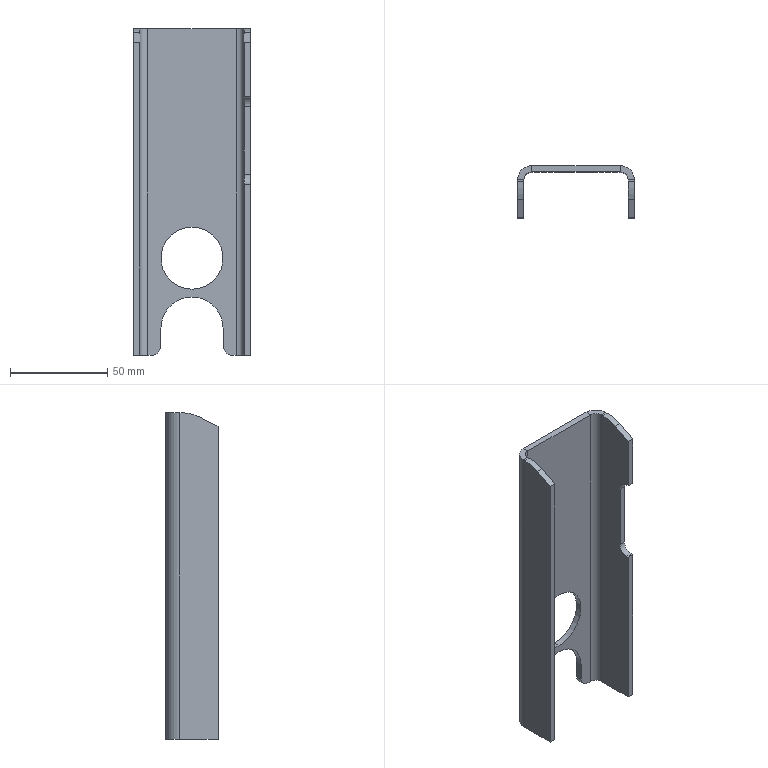Part | SolidWorks | features ICE 3, Fillet 2, FlatPattern 1, SMBaseFlange 1, SheetMetal 1, UnFold 1 | 1 solid | 41 faces | box 60 x 26.8 x 168.2 mm | volume 48634 mm3 | plane 27 | cylinder 14 | commonest cylinder face diameters 10 x4 32 x4 8 x2 14.4 x2 40 x2
STEP:
#1=CARTESIAN_POINT('',(0.,-3.2,34.));
#2=VERTEX_POINT('',#1);
#3=CARTESIAN_POINT('',(0.,-3.2,66.));
#4=VERTEX_POINT('',#3);
#5=CARTESIAN_POINT('',(0.,-3.2,50.));
#6=DIRECTION('',(0.,1.,0.));
#7=DIRECTION('',(0.,0.,1.));
#8=AXIS2_PLACEMENT_3D('',#5,#6,#7);
#9=CIRCLE('',#8,16.);
#10=EDGE_CURVE('',#2,#4,#9,.T.);
#11=ORIENTED_EDGE('',*,*,#10,.F.);
#12=CARTESIAN_POINT('',(0.,0.,34.));
#13=VERTEX_POINT('',#12);
#14=CARTESIAN_POINT('',(0.,-3.2,34.));
#15=DIRECTION('',(0.,1.,0.));
#16=VECTOR('',#15,1000.);
#17=LINE('',#14,#16);
#18=EDGE_CURVE('',#2,#13,#17,.T.);
#19=ORIENTED_EDGE('',*,*,#18,.T.);
#20=CARTESIAN_POINT('',(0.,0.,66.));
#21=VERTEX_POINT('',#20);
#22=CARTESIAN_POINT('',(0.,0.,50.));
#23=DIRECTION('',(0.,1.,0.));
#24=DIRECTION('',(0.,0.,1.));
#25=AXIS2_PLACEMENT_3D('',#22,#23,#24);
#26=CIRCLE('',#25,16.);
#27=EDGE_CURVE('',#13,#21,#26,.T.);
#28=ORIENTED_EDGE('',*,*,#27,.T.);
#29=CARTESIAN_POINT('',(0.,-3.2,66.));
#30=DIRECTION('',(0.,1.,0.));
#31=VECTOR('',#30,1000.);
#32=LINE('',#29,#31);
#33=EDGE_CURVE('',#4,#21,#32,.T.);
#34=ORIENTED_EDGE('',*,*,#33,.F.);
#35=EDGE_LOOP('',(#11,#19,#28,#34));
#36=FACE_OUTER_BOUND('',#35,.T.);
#37=CARTESIAN_POINT('',(0.,-3.2,50.));
#38=DIRECTION('',(0.,1.,0.));
#39=DIRECTION('',(0.,0.,1.));
#40=AXIS2_PLACEMENT_3D('',#37,#38,#39);
#41=CYLINDRICAL_SURFACE('',#40,16.);
#42=ADVANCED_FACE('',(#36),#41,.F.);
#43=CARTESIAN_POINT('',(0.,-3.2,30.));
#44=VERTEX_POINT('',#43);
#45=CARTESIAN_POINT('',(16.,-3.2,14.));
#46=VERTEX_POINT('',#45);
#47=CARTESIAN_POINT('',(0.,-3.2,14.));
#48=DIRECTION('',(0.,1.,0.));
#49=DIRECTION('',(0.,0.,1.));
#50=AXIS2_PLACEMENT_3D('',#47,#48,#49);
#51=CIRCLE('',#50,16.);
#52=EDGE_CURVE('',#44,#46,#51,.T.);
#53=ORIENTED_EDGE('',*,*,#52,.F.);
#54=CARTESIAN_POINT('',(0.,0.,30.));
#55=VERTEX_POINT('',#54);
#56=CARTESIAN_POINT('',(0.,-3.2,30.));
#57=DIRECTION('',(0.,1.,0.));
#58=VECTOR('',#57,1000.);
#59=LINE('',#56,#58);
#60=EDGE_CURVE('',#44,#55,#59,.T.);
#61=ORIENTED_EDGE('',*,*,#60,.T.);
#62=CARTESIAN_POINT('',(16.,0.,14.));
#63=VERTEX_POINT('',#62);
#64=CARTESIAN_POINT('',(0.,0.,14.));
#65=DIRECTION('',(0.,1.,0.));
#66=DIRECTION('',(0.,0.,1.));
#67=AXIS2_PLACEMENT_3D('',#64,#65,#66);
#68=CIRCLE('',#67,16.);
#69=EDGE_CURVE('',#55,#63,#68,.T.);
#70=ORIENTED_EDGE('',*,*,#69,.T.);
#71=CARTESIAN_POINT('',(16.,-3.2,14.));
#72=DIRECTION('',(0.,1.,0.));
#73=VECTOR('',#72,1000.);
#74=LINE('',#71,#73);
#75=EDGE_CURVE('',#46,#63,#74,.T.);
#76=ORIENTED_EDGE('',*,*,#75,.F.);
#77=EDGE_LOOP('',(#53,#61,#70,#76));
#78=FACE_OUTER_BOUND('',#77,.T.);
#79=CARTESIAN_POINT('',(0.,-3.2,14.));
#80=DIRECTION('',(0.,1.,0.));
#81=DIRECTION('',(0.,0.,1.));
#82=AXIS2_PLACEMENT_3D('',#79,#80,#81);
#83=CYLINDRICAL_SURFACE('',#82,16.);
#84=ADVANCED_FACE('',(#78),#83,.F.);
#85=CARTESIAN_POINT('',(26.8,-26.8,133.2));
#86=VERTEX_POINT('',#85);
#87=CARTESIAN_POINT('',(30.,-26.8,133.2));
#88=VERTEX_POINT('',#87);
#89=CARTESIAN_POINT('',(26.8,-26.8,133.2));
#90=DIRECTION('',(1.,0.,0.));
#91=VECTOR('',#90,1000.);
#92=LINE('',#89,#91);
#93=EDGE_CURVE('',#86,#88,#92,.T.);
#94=ORIENTED_EDGE('',*,*,#93,.T.);
#95=CARTESIAN_POINT('',(30.,-26.8,161.2));
#96=VERTEX_POINT('',#95);
#97=CARTESIAN_POINT('',(30.,-26.8,168.2));
#98=DIRECTION('',(0.,0.,-1.));
#99=VECTOR('',#98,1000.);
#100=LINE('',#97,#99);
#101=EDGE_CURVE('',#96,#88,#100,.T.);
#102=ORIENTED_EDGE('',*,*,#101,.F.);
#103=CARTESIAN_POINT('',(26.8,-26.8,161.2));
#104=VERTEX_POINT('',#103);
#105=CARTESIAN_POINT('',(-30.,-26.8,161.2));
#106=DIRECTION('',(1.,0.,0.));
#107=VECTOR('',#106,1000.);
#108=LINE('',#105,#107);
#109=EDGE_CURVE('',#104,#96,#108,.T.);
#110=ORIENTED_EDGE('',*,*,#109,.F.);
#111=CARTESIAN_POINT('',(26.8,-26.8,168.2));
#112=DIRECTION('',(0.,0.,-1.));
#113=VECTOR('',#112,1000.);
#114=LINE('',#111,#113);
#115=EDGE_CURVE('',#104,#86,#114,.T.);
#116=ORIENTED_EDGE('',*,*,#115,.T.);
#117=EDGE_LOOP('',(#94,#102,#110,#116));
#118=FACE_OUTER_BOUND('',#117,.T.);
#119=CARTESIAN_POINT('',(30.,-26.8,168.2));
#120=DIRECTION('',(0.,-1.,0.));
#121=DIRECTION('',(0.,0.,-1.));
#122=AXIS2_PLACEMENT_3D('',#119,#120,#121);
#123=PLANE('',#122);
#124=ADVANCED_FACE('',(#118),#123,.T.);
#125=CARTESIAN_POINT('',(-21.,0.,0.));
#126=VERTEX_POINT('',#125);
#127=CARTESIAN_POINT('',(-22.8,0.,0.));
#128=VERTEX_POINT('',#127);
#129=CARTESIAN_POINT('',(-30.,0.,0.));
#130=DIRECTION('',(-1.,0.,0.));
#131=VECTOR('',#130,1000.);
#132=LINE('',#129,#131);
#133=EDGE_CURVE('',#126,#128,#132,.T.);
#134=ORIENTED_EDGE('',*,*,#133,.F.);
#135=CARTESIAN_POINT('',(-21.,-3.2,0.));
#136=VERTEX_POINT('',#135);
#137=CARTESIAN_POINT('',(-21.,-3.2,0.));
#138=DIRECTION('',(0.,-1.,0.));
#139=VECTOR('',#138,1000.);
#140=LINE('',#137,#139);
#141=EDGE_CURVE('',#126,#136,#140,.T.);
#142=ORIENTED_EDGE('',*,*,#141,.T.);
#143=CARTESIAN_POINT('',(-22.8,-3.2,0.));
#144=VERTEX_POINT('',#143);
#145=CARTESIAN_POINT('',(-30.,-3.2,0.));
#146=DIRECTION('',(-1.,0.,0.));
#147=VECTOR('',#146,1000.);
#148=LINE('',#145,#147);
#149=EDGE_CURVE('',#136,#144,#148,.T.);
#150=ORIENTED_EDGE('',*,*,#149,.T.);
#151=CARTESIAN_POINT('',(-22.8,-3.2,0.));
#152=DIRECTION('',(0.,1.,0.));
#153=VECTOR('',#152,1000.);
#154=LINE('',#151,#153);
#155=EDGE_CURVE('',#144,#128,#154,.T.);
#156=ORIENTED_EDGE('',*,*,#155,.T.);
#157=EDGE_LOOP('',(#134,#142,#150,#156));
#158=FACE_OUTER_BOUND('',#157,.T.);
#159=CARTESIAN_POINT('',(26.8,-7.2,0.));
#160=DIRECTION('',(0.,0.,-1.));
#161=DIRECTION('',(-1.,0.,0.));
#162=AXIS2_PLACEMENT_3D('',#159,#160,#161);
#163=PLANE('',#162);
#164=ADVANCED_FACE('',(#158),#163,.T.);
#165=CARTESIAN_POINT('',(30.,-7.2,168.2));
#166=VERTEX_POINT('',#165);
#167=CARTESIAN_POINT('',(26.8,-7.2,168.2));
#168=VERTEX_POINT('',#167);
#169=CARTESIAN_POINT('',(30.,-7.2,168.2));
#170=DIRECTION('',(-1.,0.,0.));
#171=VECTOR('',#170,1000.);
#172=LINE('',#169,#171);
#173=EDGE_CURVE('',#166,#168,#172,.T.);
#174=ORIENTED_EDGE('',*,*,#173,.F.);
#175=CARTESIAN_POINT('',(22.8,0.,168.2));
#176=VERTEX_POINT('',#175);
#177=CARTESIAN_POINT('',(22.8,-7.2,168.2));
#178=DIRECTION('',(0.,0.,1.));
#179=DIRECTION('',(-1.,0.,0.));
#180=AXIS2_PLACEMENT_3D('',#177,#178,#179);
#181=CIRCLE('',#180,7.2);
#182=EDGE_CURVE('',#166,#176,#181,.T.);
#183=ORIENTED_EDGE('',*,*,#182,.T.);
#184=CARTESIAN_POINT('',(22.8,-3.2,168.2));
#185=VERTEX_POINT('',#184);
#186=CARTESIAN_POINT('',(22.8,-3.2,168.2));
#187=DIRECTION('',(0.,1.,0.));
#188=VECTOR('',#187,1000.);
#189=LINE('',#186,#188);
#190=EDGE_CURVE('',#185,#176,#189,.T.);
#191=ORIENTED_EDGE('',*,*,#190,.F.);
#192=CARTESIAN_POINT('',(22.8,-7.2,168.2));
#193=DIRECTION('',(0.,0.,1.));
#194=DIRECTION('',(1.,0.,0.));
#195=AXIS2_PLACEMENT_3D('',#192,#193,#194);
#196=CIRCLE('',#195,4.);
#197=EDGE_CURVE('',#168,#185,#196,.T.);
#198=ORIENTED_EDGE('',*,*,#197,.F.);
#199=EDGE_LOOP('',(#174,#183,#191,#198));
#200=FACE_OUTER_BOUND('',#199,.T.);
#201=CARTESIAN_POINT('',(30.,-7.2,168.2));
#202=DIRECTION('',(0.,0.,1.));
#203=DIRECTION('',(1.,0.,0.));
#204=AXIS2_PLACEMENT_3D('',#201,#202,#203);
#205=PLANE('',#204);
#206=ADVANCED_FACE('',(#200),#205,.T.);
#207=CARTESIAN_POINT('',(26.8,-8.218,168.2));
#208=VERTEX_POINT('',#207);
#209=CARTESIAN_POINT('',(26.8,0.,168.2));
#210=DIRECTION('',(0.,1.,0.));
#211=VECTOR('',#210,1000.);
#212=LINE('',#209,#211);
#213=EDGE_CURVE('',#208,#168,#212,.T.);
#214=ORIENTED_EDGE('',*,*,#213,.F.);
#215=CARTESIAN_POINT('',(30.,-8.218,168.2));
#216=VERTEX_POINT('',#215);
#217=CARTESIAN_POINT('',(30.,-8.218,168.2));
#218=DIRECTION('',(1.,0.,0.));
#219=VECTOR('',#218,1000.);
#220=LINE('',#217,#219);
#221=EDGE_CURVE('',#208,#216,#220,.T.);
#222=ORIENTED_EDGE('',*,*,#221,.T.);
#223=CARTESIAN_POINT('',(30.,0.,168.2));
#224=DIRECTION('',(0.,1.,0.));
#225=VECTOR('',#224,1000.);
#226=LINE('',#223,#225);
#227=EDGE_CURVE('',#216,#166,#226,.T.);
#228=ORIENTED_EDGE('',*,*,#227,.T.);
#229=ORIENTED_EDGE('',*,*,#173,.T.);
#230=EDGE_LOOP('',(#214,#222,#228,#229));
#231=FACE_OUTER_BOUND('',#230,.T.);
#232=CARTESIAN_POINT('',(22.8,-3.2,168.2));
#233=DIRECTION('',(0.,0.,1.));
#234=DIRECTION('',(1.,0.,0.));
#235=AXIS2_PLACEMENT_3D('',#232,#233,#234);
#236=PLANE('',#235);
#237=ADVANCED_FACE('',(#231),#236,.T.);
#238=CARTESIAN_POINT('',(22.8,0.,0.));
#239=VERTEX_POINT('',#238);
#240=CARTESIAN_POINT('',(22.8,-3.2,0.));
#241=VERTEX_POINT('',#240);
#242=CARTESIAN_POINT('',(22.8,0.,0.));
#243=DIRECTION('',(0.,-1.,0.));
#244=VECTOR('',#243,1000.);
#245=LINE('',#242,#244);
#246=EDGE_CURVE('',#239,#241,#245,.T.);
#247=ORIENTED_EDGE('',*,*,#246,.F.);
#248=CARTESIAN_POINT('',(30.,-7.2,0.));
#249=VERTEX_POINT('',#248);
#250=CARTESIAN_POINT('',(22.8,-7.2,0.));
#251=DIRECTION('',(0.,0.,1.));
#252=DIRECTION('',(-1.,0.,0.));
#253=AXIS2_PLACEMENT_3D('',#250,#251,#252);
#254=CIRCLE('',#253,7.2);
#255=EDGE_CURVE('',#249,#239,#254,.T.);
#256=ORIENTED_EDGE('',*,*,#255,.F.);
#257=CARTESIAN_POINT('',(26.8,-7.2,0.));
#258=VERTEX_POINT('',#257);
#259=CARTESIAN_POINT('',(26.8,-7.2,0.));
#260=DIRECTION('',(1.,0.,0.));
#261=VECTOR('',#260,1000.);
#262=LINE('',#259,#261);
#263=EDGE_CURVE('',#258,#249,#262,.T.);
#264=ORIENTED_EDGE('',*,*,#263,.F.);
#265=CARTESIAN_POINT('',(22.8,-7.2,0.));
#266=DIRECTION('',(0.,0.,1.));
#267=DIRECTION('',(1.,0.,0.));
#268=AXIS2_PLACEMENT_3D('',#265,#266,#267);
#269=CIRCLE('',#268,4.);
#270=EDGE_CURVE('',#258,#241,#269,.T.);
#271=ORIENTED_EDGE('',*,*,#270,.T.);
#272=EDGE_LOOP('',(#247,#256,#264,#271));
#273=FACE_OUTER_BOUND('',#272,.T.);
#274=CARTESIAN_POINT('',(22.8,0.,0.));
#275=DIRECTION('',(0.,0.,-1.));
#276=DIRECTION('',(-1.,0.,0.));
#277=AXIS2_PLACEMENT_3D('',#274,#275,#276);
#278=PLANE('',#277);
#279=ADVANCED_FACE('',(#273),#278,.T.);
#280=CARTESIAN_POINT('',(21.,-3.2,0.));
#281=VERTEX_POINT('',#280);
#282=CARTESIAN_POINT('',(-30.,-3.2,0.));
#283=DIRECTION('',(-1.,0.,0.));
#284=VECTOR('',#283,1000.);
#285=LINE('',#282,#284);
#286=EDGE_CURVE('',#241,#281,#285,.T.);
#287=ORIENTED_EDGE('',*,*,#286,.T.);
#288=CARTESIAN_POINT('',(21.,0.,0.));
#289=VERTEX_POINT('',#288);
#290=CARTESIAN_POINT('',(21.,0.,0.));
#291=DIRECTION('',(0.,1.,0.));
#292=VECTOR('',#291,1000.);
#293=LINE('',#290,#292);
#294=EDGE_CURVE('',#281,#289,#293,.T.);
#295=ORIENTED_EDGE('',*,*,#294,.T.);
#296=CARTESIAN_POINT('',(-30.,0.,0.));
#297=DIRECTION('',(-1.,0.,0.));
#298=VECTOR('',#297,1000.);
#299=LINE('',#296,#298);
#300=EDGE_CURVE('',#239,#289,#299,.T.);
#301=ORIENTED_EDGE('',*,*,#300,.F.);
#302=ORIENTED_EDGE('',*,*,#246,.T.);
#303=EDGE_LOOP('',(#287,#295,#301,#302));
#304=FACE_OUTER_BOUND('',#303,.T.);
#305=CARTESIAN_POINT('',(26.8,-7.2,0.));
#306=DIRECTION('',(0.,0.,-1.));
#307=DIRECTION('',(-1.,0.,0.));
#308=AXIS2_PLACEMENT_3D('',#305,#306,#307);
#309=PLANE('',#308);
#310=ADVANCED_FACE('',(#304),#309,.T.);
#311=CARTESIAN_POINT('',(-22.8,0.,168.2));
#312=VERTEX_POINT('',#311);
#313=CARTESIAN_POINT('',(-22.8,-3.2,168.2));
#314=VERTEX_POINT('',#313);
#315=CARTESIAN_POINT('',(-22.8,0.,168.2));
#316=DIRECTION('',(0.,-1.,0.));
#317=VECTOR('',#316,1000.);
#318=LINE('',#315,#317);
#319=EDGE_CURVE('',#312,#314,#318,.T.);
#320=ORIENTED_EDGE('',*,*,#319,.F.);
#321=CARTESIAN_POINT('',(-30.,-7.2,168.2));
#322=VERTEX_POINT('',#321);
#323=CARTESIAN_POINT('',(-22.8,-7.2,168.2));
#324=DIRECTION('',(0.,0.,1.));
#325=DIRECTION('',(-1.,0.,0.));
#326=AXIS2_PLACEMENT_3D('',#323,#324,#325);
#327=CIRCLE('',#326,7.2);
#328=EDGE_CURVE('',#312,#322,#327,.T.);
#329=ORIENTED_EDGE('',*,*,#328,.T.);
#330=CARTESIAN_POINT('',(-26.8,-7.2,168.2));
#331=VERTEX_POINT('',#330);
#332=CARTESIAN_POINT('',(-26.8,-7.2,168.2));
#333=DIRECTION('',(-1.,0.,0.));
#334=VECTOR('',#333,1000.);
#335=LINE('',#332,#334);
#336=EDGE_CURVE('',#331,#322,#335,.T.);
#337=ORIENTED_EDGE('',*,*,#336,.F.);
#338=CARTESIAN_POINT('',(-22.8,-7.2,168.2));
#339=DIRECTION('',(0.,0.,1.));
#340=DIRECTION('',(1.,0.,0.));
#341=AXIS2_PLACEMENT_3D('',#338,#339,#340);
#342=CIRCLE('',#341,4.);
#343=EDGE_CURVE('',#314,#331,#342,.T.);
#344=ORIENTED_EDGE('',*,*,#343,.F.);
#345=EDGE_LOOP('',(#320,#329,#337,#344));
#346=FACE_OUTER_BOUND('',#345,.T.);
#347=CARTESIAN_POINT('',(-22.8,0.,168.2));
#348=DIRECTION('',(0.,0.,1.));
#349=DIRECTION('',(1.,0.,0.));
#350=AXIS2_PLACEMENT_3D('',#347,#348,#349);
#351=PLANE('',#350);
#352=ADVANCED_FACE('',(#346),#351,.T.);
#353=CARTESIAN_POINT('',(-30.,0.,168.2));
#354=DIRECTION('',(-1.,0.,0.));
#355=VECTOR('',#354,1000.);
#356=LINE('',#353,#355);
#357=EDGE_CURVE('',#176,#312,#356,.T.);
#358=ORIENTED_EDGE('',*,*,#357,.T.);
#359=ORIENTED_EDGE('',*,*,#319,.T.);
#360=CARTESIAN_POINT('',(-30.,-3.2,168.2));
#361=DIRECTION('',(-1.,0.,0.));
#362=VECTOR('',#361,1000.);
#363=LINE('',#360,#362);
#364=EDGE_CURVE('',#185,#314,#363,.T.);
#365=ORIENTED_EDGE('',*,*,#364,.F.);
#366=ORIENTED_EDGE('',*,*,#190,.T.);
#367=EDGE_LOOP('',(#358,#359,#365,#366));
#368=FACE_OUTER_BOUND('',#367,.T.);
#369=CARTESIAN_POINT('',(-26.8,-7.2,168.2));
#370=DIRECTION('',(0.,0.,1.));
#371=DIRECTION('',(1.,0.,0.));
#372=AXIS2_PLACEMENT_3D('',#369,#370,#371);
#373=PLANE('',#372);
#374=ADVANCED_FACE('',(#368),#373,.T.);
#375=CARTESIAN_POINT('',(-30.,-7.2,0.));
#376=VERTEX_POINT('',#375);
#377=CARTESIAN_POINT('',(-26.8,-7.2,0.));
#378=VERTEX_POINT('',#377);
#379=CARTESIAN_POINT('',(-30.,-7.2,0.));
#380=DIRECTION('',(1.,0.,0.));
#381=VECTOR('',#380,1000.);
#382=LINE('',#379,#381);
#383=EDGE_CURVE('',#376,#378,#382,.T.);
#384=ORIENTED_EDGE('',*,*,#383,.F.);
#385=CARTESIAN_POINT('',(-22.8,-7.2,0.));
#386=DIRECTION('',(0.,0.,1.));
#387=DIRECTION('',(-1.,0.,0.));
#388=AXIS2_PLACEMENT_3D('',#385,#386,#387);
#389=CIRCLE('',#388,7.2);
#390=EDGE_CURVE('',#128,#376,#389,.T.);
#391=ORIENTED_EDGE('',*,*,#390,.F.);
#392=ORIENTED_EDGE('',*,*,#155,.F.);
#393=CARTESIAN_POINT('',(-22.8,-7.2,0.));
#394=DIRECTION('',(0.,0.,1.));
#395=DIRECTION('',(1.,0.,0.));
#396=AXIS2_PLACEMENT_3D('',#393,#394,#395);
#397=CIRCLE('',#396,4.);
#398=EDGE_CURVE('',#144,#378,#397,.T.);
#399=ORIENTED_EDGE('',*,*,#398,.T.);
#400=EDGE_LOOP('',(#384,#391,#392,#399));
#401=FACE_OUTER_BOUND('',#400,.T.);
#402=CARTESIAN_POINT('',(-30.,-7.2,0.));
#403=DIRECTION('',(0.,0.,-1.));
#404=DIRECTION('',(-1.,0.,0.));
#405=AXIS2_PLACEMENT_3D('',#402,#403,#404);
#406=PLANE('',#405);
#407=ADVANCED_FACE('',(#401),#406,.T.);
#408=CARTESIAN_POINT('',(-30.,-26.8,0.));
#409=VERTEX_POINT('',#408);
#410=CARTESIAN_POINT('',(-30.,0.,0.));
#411=DIRECTION('',(0.,-1.,0.));
#412=VECTOR('',#411,1000.);
#413=LINE('',#410,#412);
#414=EDGE_CURVE('',#376,#409,#413,.T.);
#415=ORIENTED_EDGE('',*,*,#414,.F.);
#416=ORIENTED_EDGE('',*,*,#383,.T.);
#417=CARTESIAN_POINT('',(-26.8,-26.8,0.));
#418=VERTEX_POINT('',#417);
#419=CARTESIAN_POINT('',(-26.8,0.,0.));
#420=DIRECTION('',(0.,-1.,0.));
#421=VECTOR('',#420,1000.);
#422=LINE('',#419,#421);
#423=EDGE_CURVE('',#378,#418,#422,.T.);
#424=ORIENTED_EDGE('',*,*,#423,.T.);
#425=CARTESIAN_POINT('',(-26.8,-26.8,0.));
#426=DIRECTION('',(-1.,0.,0.));
#427=VECTOR('',#426,1000.);
#428=LINE('',#425,#427);
#429=EDGE_CURVE('',#418,#409,#428,.T.);
#430=ORIENTED_EDGE('',*,*,#429,.T.);
#431=EDGE_LOOP('',(#415,#416,#424,#430));
#432=FACE_OUTER_BOUND('',#431,.T.);
#433=CARTESIAN_POINT('',(-22.8,-3.2,0.));
#434=DIRECTION('',(0.,0.,-1.));
#435=DIRECTION('',(-1.,0.,0.));
#436=AXIS2_PLACEMENT_3D('',#433,#434,#435);
#437=PLANE('',#436);
#438=ADVANCED_FACE('',(#432),#437,.T.);
#439=CARTESIAN_POINT('',(-30.,-26.8,161.2));
#440=VERTEX_POINT('',#439);
#441=CARTESIAN_POINT('',(-30.,-17.265,166.037));
#442=VERTEX_POINT('',#441);
#443=CARTESIAN_POINT('',(-30.,-26.8,161.2));
#444=DIRECTION('',(0.,0.8918,0.4524));
#445=VECTOR('',#444,1000.);
#446=LINE('',#443,#445);
#447=EDGE_CURVE('',#440,#442,#446,.T.);
#448=ORIENTED_EDGE('',*,*,#447,.T.);
#449=CARTESIAN_POINT('',(-30.,-8.218,168.2));
#450=VERTEX_POINT('',#449);
#451=CARTESIAN_POINT('',(-30.,-8.218,148.2));
#452=DIRECTION('',(-1.,0.,0.));
#453=DIRECTION('',(0.,0.,-1.));
#454=AXIS2_PLACEMENT_3D('',#451,#452,#453);
#455=CIRCLE('',#454,20.);
#456=EDGE_CURVE('',#442,#450,#455,.T.);
#457=ORIENTED_EDGE('',*,*,#456,.T.);
#458=CARTESIAN_POINT('',(-30.,0.,168.2));
#459=DIRECTION('',(0.,-1.,0.));
#460=VECTOR('',#459,1000.);
#461=LINE('',#458,#460);
#462=EDGE_CURVE('',#322,#450,#461,.T.);
#463=ORIENTED_EDGE('',*,*,#462,.F.);
#464=CARTESIAN_POINT('',(-30.,-7.2,168.2));
#465=DIRECTION('',(0.,0.,-1.));
#466=VECTOR('',#465,1000.);
#467=LINE('',#464,#466);
#468=EDGE_CURVE('',#322,#376,#467,.T.);
#469=ORIENTED_EDGE('',*,*,#468,.T.);
#470=ORIENTED_EDGE('',*,*,#414,.T.);
#471=CARTESIAN_POINT('',(-30.,-26.8,168.2));
#472=DIRECTION('',(0.,0.,-1.));
#473=VECTOR('',#472,1000.);
#474=LINE('',#471,#473);
#475=EDGE_CURVE('',#440,#409,#474,.T.);
#476=ORIENTED_EDGE('',*,*,#475,.F.);
#477=EDGE_LOOP('',(#448,#457,#463,#469,#470,#476));
#478=FACE_OUTER_BOUND('',#477,.T.);
#479=CARTESIAN_POINT('',(-30.,0.,168.2));
#480=DIRECTION('',(1.,0.,0.));
#481=DIRECTION('',(0.,0.,-1.));
#482=AXIS2_PLACEMENT_3D('',#479,#480,#481);
#483=PLANE('',#482);
#484=ADVANCED_FACE('',(#478),#483,.F.);
#485=CARTESIAN_POINT('',(-26.8,-26.8,161.2));
#486=VERTEX_POINT('',#485);
#487=CARTESIAN_POINT('',(-30.,-26.8,161.2));
#488=DIRECTION('',(1.,0.,0.));
#489=VECTOR('',#488,1000.);
#490=LINE('',#487,#489);
#491=EDGE_CURVE('',#440,#486,#490,.T.);
#492=ORIENTED_EDGE('',*,*,#491,.F.);
#493=ORIENTED_EDGE('',*,*,#475,.T.);
#494=ORIENTED_EDGE('',*,*,#429,.F.);
#495=CARTESIAN_POINT('',(-26.8,-26.8,168.2));
#496=DIRECTION('',(0.,0.,-1.));
#497=VECTOR('',#496,1000.);
#498=LINE('',#495,#497);
#499=EDGE_CURVE('',#486,#418,#498,.T.);
#500=ORIENTED_EDGE('',*,*,#499,.F.);
#501=EDGE_LOOP('',(#492,#493,#494,#500));
#502=FACE_OUTER_BOUND('',#501,.T.);
#503=CARTESIAN_POINT('',(-26.8,-26.8,168.2));
#504=DIRECTION('',(0.,-1.,0.));
#505=DIRECTION('',(0.,0.,-1.));
#506=AXIS2_PLACEMENT_3D('',#503,#504,#505);
#507=PLANE('',#506);
#508=ADVANCED_FACE('',(#502),#507,.T.);
#509=CARTESIAN_POINT('',(-26.8,-8.218,168.2));
#510=VERTEX_POINT('',#509);
#511=CARTESIAN_POINT('',(-26.8,0.,168.2));
#512=DIRECTION('',(0.,-1.,0.));
#513=VECTOR('',#512,1000.);
#514=LINE('',#511,#513);
#515=EDGE_CURVE('',#331,#510,#514,.T.);
#516=ORIENTED_EDGE('',*,*,#515,.T.);
#517=CARTESIAN_POINT('',(-26.8,-17.265,166.037));
#518=VERTEX_POINT('',#517);
#519=CARTESIAN_POINT('',(-26.8,-8.218,148.2));
#520=DIRECTION('',(1.,0.,0.));
#521=DIRECTION('',(0.,0.,-1.));
#522=AXIS2_PLACEMENT_3D('',#519,#520,#521);
#523=CIRCLE('',#522,20.);
#524=EDGE_CURVE('',#510,#518,#523,.T.);
#525=ORIENTED_EDGE('',*,*,#524,.T.);
#526=CARTESIAN_POINT('',(-26.8,-2.66,173.445));
#527=DIRECTION('',(0.,0.8918,0.4524));
#528=VECTOR('',#527,1000.);
#529=LINE('',#526,#528);
#530=EDGE_CURVE('',#486,#518,#529,.T.);
#531=ORIENTED_EDGE('',*,*,#530,.F.);
#532=ORIENTED_EDGE('',*,*,#499,.T.);
#533=ORIENTED_EDGE('',*,*,#423,.F.);
#534=CARTESIAN_POINT('',(-26.8,-7.2,168.2));
#535=DIRECTION('',(0.,0.,-1.));
#536=VECTOR('',#535,1000.);
#537=LINE('',#534,#536);
#538=EDGE_CURVE('',#331,#378,#537,.T.);
#539=ORIENTED_EDGE('',*,*,#538,.F.);
#540=EDGE_LOOP('',(#516,#525,#531,#532,#533,#539));
#541=FACE_OUTER_BOUND('',#540,.T.);
#542=CARTESIAN_POINT('',(-26.8,0.,168.2));
#543=DIRECTION('',(1.,0.,0.));
#544=DIRECTION('',(0.,0.,-1.));
#545=AXIS2_PLACEMENT_3D('',#542,#543,#544);
#546=PLANE('',#545);
#547=ADVANCED_FACE('',(#541),#546,.T.);
#548=ORIENTED_EDGE('',*,*,#398,.F.);
#549=CARTESIAN_POINT('',(-22.8,-3.2,168.2));
#550=DIRECTION('',(0.,0.,-1.));
#551=VECTOR('',#550,1000.);
#552=LINE('',#549,#551);
#553=EDGE_CURVE('',#314,#144,#552,.T.);
#554=ORIENTED_EDGE('',*,*,#553,.F.);
#555=ORIENTED_EDGE('',*,*,#343,.T.);
#556=ORIENTED_EDGE('',*,*,#538,.T.);
#557=EDGE_LOOP('',(#548,#554,#555,#556));
#558=FACE_OUTER_BOUND('',#557,.T.);
#559=CARTESIAN_POINT('',(-22.8,-7.2,168.2));
#560=DIRECTION('',(0.,0.,-1.));
#561=DIRECTION('',(-1.,0.,0.));
#562=AXIS2_PLACEMENT_3D('',#559,#560,#561);
#563=CYLINDRICAL_SURFACE('',#562,4.);
#564=ADVANCED_FACE('',(#558),#563,.F.);
#565=CARTESIAN_POINT('',(0.,-3.2,50.));
#566=DIRECTION('',(0.,1.,0.));
#567=DIRECTION('',(0.,0.,1.));
#568=AXIS2_PLACEMENT_3D('',#565,#566,#567);
#569=CIRCLE('',#568,16.);
#570=EDGE_CURVE('',#4,#2,#569,.T.);
#571=ORIENTED_EDGE('',*,*,#570,.T.);
#572=ORIENTED_EDGE('',*,*,#10,.T.);
#573=EDGE_LOOP('',(#571,#572));
#574=FACE_BOUND('',#573,.T.);
#575=CARTESIAN_POINT('',(16.,-3.2,5.));
#576=VERTEX_POINT('',#575);
#577=CARTESIAN_POINT('',(16.,-3.2,14.));
#578=DIRECTION('',(0.,0.,-1.));
#579=VECTOR('',#578,1000.);
#580=LINE('',#577,#579);
#581=EDGE_CURVE('',#46,#576,#580,.T.);
#582=ORIENTED_EDGE('',*,*,#581,.T.);
#583=CARTESIAN_POINT('',(21.,-3.2,5.));
#584=DIRECTION('',(0.,-1.,0.));
#585=DIRECTION('',(0.,0.,-1.));
#586=AXIS2_PLACEMENT_3D('',#583,#584,#585);
#587=CIRCLE('',#586,5.);
#588=EDGE_CURVE('',#576,#281,#587,.T.);
#589=ORIENTED_EDGE('',*,*,#588,.T.);
#590=ORIENTED_EDGE('',*,*,#286,.F.);
#591=CARTESIAN_POINT('',(22.8,-3.2,168.2));
#592=DIRECTION('',(0.,0.,-1.));
#593=VECTOR('',#592,1000.);
#594=LINE('',#591,#593);
#595=EDGE_CURVE('',#185,#241,#594,.T.);
#596=ORIENTED_EDGE('',*,*,#595,.F.);
#597=ORIENTED_EDGE('',*,*,#364,.T.);
#598=ORIENTED_EDGE('',*,*,#553,.T.);
#599=ORIENTED_EDGE('',*,*,#149,.F.);
#600=CARTESIAN_POINT('',(-16.,-3.2,5.));
#601=VERTEX_POINT('',#600);
#602=CARTESIAN_POINT('',(-21.,-3.2,5.));
#603=DIRECTION('',(0.,-1.,0.));
#604=DIRECTION('',(0.,0.,-1.));
#605=AXIS2_PLACEMENT_3D('',#602,#603,#604);
#606=CIRCLE('',#605,5.);
#607=EDGE_CURVE('',#136,#601,#606,.T.);
#608=ORIENTED_EDGE('',*,*,#607,.T.);
#609=CARTESIAN_POINT('',(-16.,-3.2,14.));
#610=VERTEX_POINT('',#609);
#611=CARTESIAN_POINT('',(-16.,-3.2,14.));
#612=DIRECTION('',(0.,0.,1.));
#613=VECTOR('',#612,1000.);
#614=LINE('',#611,#613);
#615=EDGE_CURVE('',#601,#610,#614,.T.);
#616=ORIENTED_EDGE('',*,*,#615,.T.);
#617=CARTESIAN_POINT('',(0.,-3.2,14.));
#618=DIRECTION('',(0.,1.,0.));
#619=DIRECTION('',(0.,0.,1.));
#620=AXIS2_PLACEMENT_3D('',#617,#618,#619);
#621=CIRCLE('',#620,16.);
#622=EDGE_CURVE('',#610,#44,#621,.T.);
#623=ORIENTED_EDGE('',*,*,#622,.T.);
#624=ORIENTED_EDGE('',*,*,#52,.T.);
#625=EDGE_LOOP('',(#582,#589,#590,#596,#597,#598,#599,#608,#616,#623,#624));
#626=FACE_OUTER_BOUND('',#625,.T.);
#627=CARTESIAN_POINT('',(-30.,-3.2,168.2));
#628=DIRECTION('',(0.,-1.,0.));
#629=DIRECTION('',(0.,0.,-1.));
#630=AXIS2_PLACEMENT_3D('',#627,#628,#629);
#631=PLANE('',#630);
#632=ADVANCED_FACE('',(#574,#626),#631,.T.);
#633=ORIENTED_EDGE('',*,*,#270,.F.);
#634=CARTESIAN_POINT('',(26.8,-7.2,168.2));
#635=DIRECTION('',(0.,0.,-1.));
#636=VECTOR('',#635,1000.);
#637=LINE('',#634,#636);
#638=EDGE_CURVE('',#168,#258,#637,.T.);
#639=ORIENTED_EDGE('',*,*,#638,.F.);
#640=ORIENTED_EDGE('',*,*,#197,.T.);
#641=ORIENTED_EDGE('',*,*,#595,.T.);
#642=EDGE_LOOP('',(#633,#639,#640,#641));
#643=FACE_OUTER_BOUND('',#642,.T.);
#644=CARTESIAN_POINT('',(22.8,-7.2,168.2));
#645=DIRECTION('',(0.,0.,-1.));
#646=DIRECTION('',(-1.,0.,0.));
#647=AXIS2_PLACEMENT_3D('',#644,#645,#646);
#648=CYLINDRICAL_SURFACE('',#647,4.);
#649=ADVANCED_FACE('',(#643),#648,.F.);
#650=CARTESIAN_POINT('',(26.8,-25.8,133.2));
#651=VERTEX_POINT('',#650);
#652=CARTESIAN_POINT('',(26.8,-26.8,133.2));
#653=DIRECTION('',(0.,-1.,0.));
#654=VECTOR('',#653,1000.);
#655=LINE('',#652,#654);
#656=EDGE_CURVE('',#651,#86,#655,.T.);
#657=ORIENTED_EDGE('',*,*,#656,.T.);
#658=ORIENTED_EDGE('',*,*,#115,.F.);
#659=CARTESIAN_POINT('',(26.8,-17.265,166.037));
#660=VERTEX_POINT('',#659);
#661=CARTESIAN_POINT('',(26.8,-2.66,173.445));
#662=DIRECTION('',(0.,-0.8918,-0.4524));
#663=VECTOR('',#662,1000.);
#664=LINE('',#661,#663);
#665=EDGE_CURVE('',#660,#104,#664,.T.);
#666=ORIENTED_EDGE('',*,*,#665,.F.);
#667=CARTESIAN_POINT('',(26.8,-8.218,148.2));
#668=DIRECTION('',(-1.,0.,0.));
#669=DIRECTION('',(0.,-1.,0.));
#670=AXIS2_PLACEMENT_3D('',#667,#668,#669);
#671=CIRCLE('',#670,20.);
#672=EDGE_CURVE('',#660,#208,#671,.T.);
#673=ORIENTED_EDGE('',*,*,#672,.T.);
#674=ORIENTED_EDGE('',*,*,#213,.T.);
#675=ORIENTED_EDGE('',*,*,#638,.T.);
#676=CARTESIAN_POINT('',(26.8,-26.8,0.));
#677=VERTEX_POINT('',#676);
#678=CARTESIAN_POINT('',(26.8,0.,0.));
#679=DIRECTION('',(0.,1.,0.));
#680=VECTOR('',#679,1000.);
#681=LINE('',#678,#680);
#682=EDGE_CURVE('',#677,#258,#681,.T.);
#683=ORIENTED_EDGE('',*,*,#682,.F.);
#684=CARTESIAN_POINT('',(26.8,-26.8,88.2));
#685=VERTEX_POINT('',#684);
#686=CARTESIAN_POINT('',(26.8,-26.8,168.2));
#687=DIRECTION('',(0.,0.,-1.));
#688=VECTOR('',#687,1000.);
#689=LINE('',#686,#688);
#690=EDGE_CURVE('',#685,#677,#689,.T.);
#691=ORIENTED_EDGE('',*,*,#690,.F.);
#692=CARTESIAN_POINT('',(26.8,-25.8,88.2));
#693=VERTEX_POINT('',#692);
#694=CARTESIAN_POINT('',(26.8,-25.8,88.2));
#695=DIRECTION('',(0.,1.,0.));
#696=VECTOR('',#695,1000.);
#697=LINE('',#694,#696);
#698=EDGE_CURVE('',#685,#693,#697,.T.);
#699=ORIENTED_EDGE('',*,*,#698,.T.);
#700=CARTESIAN_POINT('',(26.8,-20.8,93.2));
#701=VERTEX_POINT('',#700);
#702=CARTESIAN_POINT('',(26.8,-25.8,93.2));
#703=DIRECTION('',(1.,0.,0.));
#704=DIRECTION('',(0.,-1.,0.));
#705=AXIS2_PLACEMENT_3D('',#702,#703,#704);
#706=CIRCLE('',#705,5.);
#707=EDGE_CURVE('',#693,#701,#706,.T.);
#708=ORIENTED_EDGE('',*,*,#707,.T.);
#709=CARTESIAN_POINT('',(26.8,-20.8,128.2));
#710=VERTEX_POINT('',#709);
#711=CARTESIAN_POINT('',(26.8,-20.8,128.2));
#712=DIRECTION('',(0.,0.,1.));
#713=VECTOR('',#712,1000.);
#714=LINE('',#711,#713);
#715=EDGE_CURVE('',#701,#710,#714,.T.);
#716=ORIENTED_EDGE('',*,*,#715,.T.);
#717=CARTESIAN_POINT('',(26.8,-25.8,128.2));
#718=DIRECTION('',(1.,0.,0.));
#719=DIRECTION('',(0.,-1.,0.));
#720=AXIS2_PLACEMENT_3D('',#717,#718,#719);
#721=CIRCLE('',#720,5.);
#722=EDGE_CURVE('',#710,#651,#721,.T.);
#723=ORIENTED_EDGE('',*,*,#722,.T.);
#724=EDGE_LOOP('',(#657,#658,#666,#673,#674,#675,#683,#691,#699,#708,#716,#723));
#725=FACE_OUTER_BOUND('',#724,.T.);
#726=CARTESIAN_POINT('',(26.8,0.,168.2));
#727=DIRECTION('',(-1.,0.,0.));
#728=DIRECTION('',(0.,-1.,0.));
#729=AXIS2_PLACEMENT_3D('',#726,#727,#728);
#730=PLANE('',#729);
#731=ADVANCED_FACE('',(#725),#730,.T.);
#732=CARTESIAN_POINT('',(30.,-26.8,88.2));
#733=VERTEX_POINT('',#732);
#734=CARTESIAN_POINT('',(26.8,-26.8,88.2));
#735=DIRECTION('',(1.,0.,0.));
#736=VECTOR('',#735,1000.);
#737=LINE('',#734,#736);
#738=EDGE_CURVE('',#685,#733,#737,.T.);
#739=ORIENTED_EDGE('',*,*,#738,.F.);
#740=ORIENTED_EDGE('',*,*,#690,.T.);
#741=CARTESIAN_POINT('',(30.,-26.8,0.));
#742=VERTEX_POINT('',#741);
#743=CARTESIAN_POINT('',(30.,-26.8,0.));
#744=DIRECTION('',(-1.,0.,0.));
#745=VECTOR('',#744,1000.);
#746=LINE('',#743,#745);
#747=EDGE_CURVE('',#742,#677,#746,.T.);
#748=ORIENTED_EDGE('',*,*,#747,.F.);
#749=CARTESIAN_POINT('',(30.,-26.8,168.2));
#750=DIRECTION('',(0.,0.,-1.));
#751=VECTOR('',#750,1000.);
#752=LINE('',#749,#751);
#753=EDGE_CURVE('',#733,#742,#752,.T.);
#754=ORIENTED_EDGE('',*,*,#753,.F.);
#755=EDGE_LOOP('',(#739,#740,#748,#754));
#756=FACE_OUTER_BOUND('',#755,.T.);
#757=CARTESIAN_POINT('',(30.,-26.8,168.2));
#758=DIRECTION('',(0.,-1.,0.));
#759=DIRECTION('',(0.,0.,-1.));
#760=AXIS2_PLACEMENT_3D('',#757,#758,#759);
#761=PLANE('',#760);
#762=ADVANCED_FACE('',(#756),#761,.T.);
#763=ORIENTED_EDGE('',*,*,#101,.T.);
#764=CARTESIAN_POINT('',(30.,-25.8,133.2));
#765=VERTEX_POINT('',#764);
#766=CARTESIAN_POINT('',(30.,-26.8,133.2));
#767=DIRECTION('',(0.,-1.,0.));
#768=VECTOR('',#767,1000.);
#769=LINE('',#766,#768);
#770=EDGE_CURVE('',#765,#88,#769,.T.);
#771=ORIENTED_EDGE('',*,*,#770,.F.);
#772=CARTESIAN_POINT('',(30.,-20.8,128.2));
#773=VERTEX_POINT('',#772);
#774=CARTESIAN_POINT('',(30.,-25.8,128.2));
#775=DIRECTION('',(1.,0.,0.));
#776=DIRECTION('',(0.,-1.,0.));
#777=AXIS2_PLACEMENT_3D('',#774,#775,#776);
#778=CIRCLE('',#777,5.);
#779=EDGE_CURVE('',#773,#765,#778,.T.);
#780=ORIENTED_EDGE('',*,*,#779,.F.);
#781=CARTESIAN_POINT('',(30.,-20.8,93.2));
#782=VERTEX_POINT('',#781);
#783=CARTESIAN_POINT('',(30.,-20.8,128.2));
#784=DIRECTION('',(0.,0.,1.));
#785=VECTOR('',#784,1000.);
#786=LINE('',#783,#785);
#787=EDGE_CURVE('',#782,#773,#786,.T.);
#788=ORIENTED_EDGE('',*,*,#787,.F.);
#789=CARTESIAN_POINT('',(30.,-25.8,88.2));
#790=VERTEX_POINT('',#789);
#791=CARTESIAN_POINT('',(30.,-25.8,93.2));
#792=DIRECTION('',(1.,0.,0.));
#793=DIRECTION('',(0.,-1.,0.));
#794=AXIS2_PLACEMENT_3D('',#791,#792,#793);
#795=CIRCLE('',#794,5.);
#796=EDGE_CURVE('',#790,#782,#795,.T.);
#797=ORIENTED_EDGE('',*,*,#796,.F.);
#798=CARTESIAN_POINT('',(30.,-25.8,88.2));
#799=DIRECTION('',(0.,1.,0.));
#800=VECTOR('',#799,1000.);
#801=LINE('',#798,#800);
#802=EDGE_CURVE('',#733,#790,#801,.T.);
#803=ORIENTED_EDGE('',*,*,#802,.F.);
#804=ORIENTED_EDGE('',*,*,#753,.T.);
#805=CARTESIAN_POINT('',(30.,0.,0.));
#806=DIRECTION('',(0.,1.,0.));
#807=VECTOR('',#806,1000.);
#808=LINE('',#805,#807);
#809=EDGE_CURVE('',#742,#249,#808,.T.);
#810=ORIENTED_EDGE('',*,*,#809,.T.);
#811=CARTESIAN_POINT('',(30.,-7.2,168.2));
#812=DIRECTION('',(0.,0.,-1.));
#813=VECTOR('',#812,1000.);
#814=LINE('',#811,#813);
#815=EDGE_CURVE('',#166,#249,#814,.T.);
#816=ORIENTED_EDGE('',*,*,#815,.F.);
#817=ORIENTED_EDGE('',*,*,#227,.F.);
#818=CARTESIAN_POINT('',(30.,-17.265,166.037));
#819=VERTEX_POINT('',#818);
#820=CARTESIAN_POINT('',(30.,-8.218,148.2));
#821=DIRECTION('',(1.,0.,0.));
#822=DIRECTION('',(0.,-1.,0.));
#823=AXIS2_PLACEMENT_3D('',#820,#821,#822);
#824=CIRCLE('',#823,20.);
#825=EDGE_CURVE('',#216,#819,#824,.T.);
#826=ORIENTED_EDGE('',*,*,#825,.T.);
#827=CARTESIAN_POINT('',(30.,-26.8,161.2));
#828=DIRECTION('',(0.,0.8918,0.4524));
#829=VECTOR('',#828,1000.);
#830=LINE('',#827,#829);
#831=EDGE_CURVE('',#96,#819,#830,.T.);
#832=ORIENTED_EDGE('',*,*,#831,.F.);
#833=EDGE_LOOP('',(#763,#771,#780,#788,#797,#803,#804,#810,#816,#817,#826,#832));
#834=FACE_OUTER_BOUND('',#833,.T.);
#835=CARTESIAN_POINT('',(30.,0.,168.2));
#836=DIRECTION('',(-1.,0.,0.));
#837=DIRECTION('',(0.,-1.,0.));
#838=AXIS2_PLACEMENT_3D('',#835,#836,#837);
#839=PLANE('',#838);
#840=ADVANCED_FACE('',(#834),#839,.F.);
#841=ORIENTED_EDGE('',*,*,#255,.T.);
#842=CARTESIAN_POINT('',(22.8,0.,168.2));
#843=DIRECTION('',(0.,0.,-1.));
#844=VECTOR('',#843,1000.);
#845=LINE('',#842,#844);
#846=EDGE_CURVE('',#176,#239,#845,.T.);
#847=ORIENTED_EDGE('',*,*,#846,.F.);
#848=ORIENTED_EDGE('',*,*,#182,.F.);
#849=ORIENTED_EDGE('',*,*,#815,.T.);
#850=EDGE_LOOP('',(#841,#847,#848,#849));
#851=FACE_OUTER_BOUND('',#850,.T.);
#852=CARTESIAN_POINT('',(22.8,-7.2,168.2));
#853=DIRECTION('',(0.,0.,-1.));
#854=DIRECTION('',(-1.,0.,0.));
#855=AXIS2_PLACEMENT_3D('',#852,#853,#854);
#856=CYLINDRICAL_SURFACE('',#855,7.2);
#857=ADVANCED_FACE('',(#851),#856,.T.);
#858=CARTESIAN_POINT('',(0.,0.,50.));
#859=DIRECTION('',(0.,1.,0.));
#860=DIRECTION('',(0.,0.,1.));
#861=AXIS2_PLACEMENT_3D('',#858,#859,#860);
#862=CIRCLE('',#861,16.);
#863=EDGE_CURVE('',#21,#13,#862,.T.);
#864=ORIENTED_EDGE('',*,*,#863,.F.);
#865=ORIENTED_EDGE('',*,*,#27,.F.);
#866=EDGE_LOOP('',(#864,#865));
#867=FACE_BOUND('',#866,.T.);
#868=ORIENTED_EDGE('',*,*,#300,.T.);
#869=CARTESIAN_POINT('',(16.,0.,5.));
#870=VERTEX_POINT('',#869);
#871=CARTESIAN_POINT('',(21.,0.,5.));
#872=DIRECTION('',(0.,1.,0.));
#873=DIRECTION('',(0.,0.,-1.));
#874=AXIS2_PLACEMENT_3D('',#871,#872,#873);
#875=CIRCLE('',#874,5.);
#876=EDGE_CURVE('',#289,#870,#875,.T.);
#877=ORIENTED_EDGE('',*,*,#876,.T.);
#878=CARTESIAN_POINT('',(16.,0.,14.));
#879=DIRECTION('',(0.,0.,-1.));
#880=VECTOR('',#879,1000.);
#881=LINE('',#878,#880);
#882=EDGE_CURVE('',#63,#870,#881,.T.);
#883=ORIENTED_EDGE('',*,*,#882,.F.);
#884=ORIENTED_EDGE('',*,*,#69,.F.);
#885=CARTESIAN_POINT('',(-16.,0.,14.));
#886=VERTEX_POINT('',#885);
#887=CARTESIAN_POINT('',(0.,0.,14.));
#888=DIRECTION('',(0.,1.,0.));
#889=DIRECTION('',(0.,0.,1.));
#890=AXIS2_PLACEMENT_3D('',#887,#888,#889);
#891=CIRCLE('',#890,16.);
#892=EDGE_CURVE('',#886,#55,#891,.T.);
#893=ORIENTED_EDGE('',*,*,#892,.F.);
#894=CARTESIAN_POINT('',(-16.,0.,5.));
#895=VERTEX_POINT('',#894);
#896=CARTESIAN_POINT('',(-16.,0.,14.));
#897=DIRECTION('',(0.,0.,1.));
#898=VECTOR('',#897,1000.);
#899=LINE('',#896,#898);
#900=EDGE_CURVE('',#895,#886,#899,.T.);
#901=ORIENTED_EDGE('',*,*,#900,.F.);
#902=CARTESIAN_POINT('',(-21.,0.,5.));
#903=DIRECTION('',(0.,1.,0.));
#904=DIRECTION('',(0.,0.,-1.));
#905=AXIS2_PLACEMENT_3D('',#902,#903,#904);
#906=CIRCLE('',#905,5.);
#907=EDGE_CURVE('',#895,#126,#906,.T.);
#908=ORIENTED_EDGE('',*,*,#907,.T.);
#909=ORIENTED_EDGE('',*,*,#133,.T.);
#910=CARTESIAN_POINT('',(-22.8,0.,168.2));
#911=DIRECTION('',(0.,0.,-1.));
#912=VECTOR('',#911,1000.);
#913=LINE('',#910,#912);
#914=EDGE_CURVE('',#312,#128,#913,.T.);
#915=ORIENTED_EDGE('',*,*,#914,.F.);
#916=ORIENTED_EDGE('',*,*,#357,.F.);
#917=ORIENTED_EDGE('',*,*,#846,.T.);
#918=EDGE_LOOP('',(#868,#877,#883,#884,#893,#901,#908,#909,#915,#916,#917));
#919=FACE_OUTER_BOUND('',#918,.T.);
#920=CARTESIAN_POINT('',(-30.,0.,168.2));
#921=DIRECTION('',(0.,-1.,0.));
#922=DIRECTION('',(0.,0.,-1.));
#923=AXIS2_PLACEMENT_3D('',#920,#921,#922);
#924=PLANE('',#923);
#925=ADVANCED_FACE('',(#867,#919),#924,.F.);
#926=ORIENTED_EDGE('',*,*,#390,.T.);
#927=ORIENTED_EDGE('',*,*,#468,.F.);
#928=ORIENTED_EDGE('',*,*,#328,.F.);
#929=ORIENTED_EDGE('',*,*,#914,.T.);
#930=EDGE_LOOP('',(#926,#927,#928,#929));
#931=FACE_OUTER_BOUND('',#930,.T.);
#932=CARTESIAN_POINT('',(-22.8,-7.2,168.2));
#933=DIRECTION('',(0.,0.,-1.));
#934=DIRECTION('',(-1.,0.,0.));
#935=AXIS2_PLACEMENT_3D('',#932,#933,#934);
#936=CYLINDRICAL_SURFACE('',#935,7.2);
#937=ADVANCED_FACE('',(#931),#936,.T.);
#938=ORIENTED_EDGE('',*,*,#462,.T.);
#939=CARTESIAN_POINT('',(-26.8,-8.218,168.2));
#940=DIRECTION('',(1.,0.,0.));
#941=VECTOR('',#940,1000.);
#942=LINE('',#939,#941);
#943=EDGE_CURVE('',#450,#510,#942,.T.);
#944=ORIENTED_EDGE('',*,*,#943,.T.);
#945=ORIENTED_EDGE('',*,*,#515,.F.);
#946=ORIENTED_EDGE('',*,*,#336,.T.);
#947=EDGE_LOOP('',(#938,#944,#945,#946));
#948=FACE_OUTER_BOUND('',#947,.T.);
#949=CARTESIAN_POINT('',(-22.8,-7.2,168.2));
#950=DIRECTION('',(0.,0.,1.));
#951=DIRECTION('',(1.,0.,0.));
#952=AXIS2_PLACEMENT_3D('',#949,#950,#951);
#953=PLANE('',#952);
#954=ADVANCED_FACE('',(#948),#953,.T.);
#955=ORIENTED_EDGE('',*,*,#682,.T.);
#956=ORIENTED_EDGE('',*,*,#263,.T.);
#957=ORIENTED_EDGE('',*,*,#809,.F.);
#958=ORIENTED_EDGE('',*,*,#747,.T.);
#959=EDGE_LOOP('',(#955,#956,#957,#958));
#960=FACE_OUTER_BOUND('',#959,.T.);
#961=CARTESIAN_POINT('',(-22.8,-7.2,0.));
#962=DIRECTION('',(0.,0.,1.));
#963=DIRECTION('',(1.,0.,0.));
#964=AXIS2_PLACEMENT_3D('',#961,#962,#963);
#965=PLANE('',#964);
#966=ADVANCED_FACE('',(#960),#965,.F.);
#967=ORIENTED_EDGE('',*,*,#60,.F.);
#968=ORIENTED_EDGE('',*,*,#622,.F.);
#969=CARTESIAN_POINT('',(-16.,-3.2,14.));
#970=DIRECTION('',(0.,1.,0.));
#971=VECTOR('',#970,1000.);
#972=LINE('',#969,#971);
#973=EDGE_CURVE('',#610,#886,#972,.T.);
#974=ORIENTED_EDGE('',*,*,#973,.T.);
#975=ORIENTED_EDGE('',*,*,#892,.T.);
#976=EDGE_LOOP('',(#967,#968,#974,#975));
#977=FACE_OUTER_BOUND('',#976,.T.);
#978=CARTESIAN_POINT('',(0.,-3.2,14.));
#979=DIRECTION('',(0.,1.,0.));
#980=DIRECTION('',(0.,0.,1.));
#981=AXIS2_PLACEMENT_3D('',#978,#979,#980);
#982=CYLINDRICAL_SURFACE('',#981,16.);
#983=ADVANCED_FACE('',(#977),#982,.F.);
#984=ORIENTED_EDGE('',*,*,#615,.F.);
#985=CARTESIAN_POINT('',(-16.,0.,5.));
#986=DIRECTION('',(0.,1.,0.));
#987=VECTOR('',#986,1000.);
#988=LINE('',#985,#987);
#989=EDGE_CURVE('',#601,#895,#988,.T.);
#990=ORIENTED_EDGE('',*,*,#989,.T.);
#991=ORIENTED_EDGE('',*,*,#900,.T.);
#992=ORIENTED_EDGE('',*,*,#973,.F.);
#993=EDGE_LOOP('',(#984,#990,#991,#992));
#994=FACE_OUTER_BOUND('',#993,.T.);
#995=CARTESIAN_POINT('',(-16.,-3.2,14.));
#996=DIRECTION('',(-1.,0.,0.));
#997=DIRECTION('',(0.,0.,1.));
#998=AXIS2_PLACEMENT_3D('',#995,#996,#997);
#999=PLANE('',#998);
#1000=ADVANCED_FACE('',(#994),#999,.F.);
#1001=ORIENTED_EDGE('',*,*,#882,.T.);
#1002=CARTESIAN_POINT('',(16.,-3.2,5.));
#1003=DIRECTION('',(0.,-1.,0.));
#1004=VECTOR('',#1003,1000.);
#1005=LINE('',#1002,#1004);
#1006=EDGE_CURVE('',#870,#576,#1005,.T.);
#1007=ORIENTED_EDGE('',*,*,#1006,.T.);
#1008=ORIENTED_EDGE('',*,*,#581,.F.);
#1009=ORIENTED_EDGE('',*,*,#75,.T.);
#1010=EDGE_LOOP('',(#1001,#1007,#1008,#1009));
#1011=FACE_OUTER_BOUND('',#1010,.T.);
#1012=CARTESIAN_POINT('',(16.,-3.2,14.));
#1013=DIRECTION('',(1.,0.,0.));
#1014=DIRECTION('',(0.,0.,-1.));
#1015=AXIS2_PLACEMENT_3D('',#1012,#1013,#1014);
#1016=PLANE('',#1015);
#1017=ADVANCED_FACE('',(#1011),#1016,.F.);
#1018=ORIENTED_EDGE('',*,*,#18,.F.);
#1019=ORIENTED_EDGE('',*,*,#570,.F.);
#1020=ORIENTED_EDGE('',*,*,#33,.T.);
#1021=ORIENTED_EDGE('',*,*,#863,.T.);
#1022=EDGE_LOOP('',(#1018,#1019,#1020,#1021));
#1023=FACE_OUTER_BOUND('',#1022,.T.);
#1024=CARTESIAN_POINT('',(0.,-3.2,50.));
#1025=DIRECTION('',(0.,1.,0.));
#1026=DIRECTION('',(0.,0.,1.));
#1027=AXIS2_PLACEMENT_3D('',#1024,#1025,#1026);
#1028=CYLINDRICAL_SURFACE('',#1027,16.);
#1029=ADVANCED_FACE('',(#1023),#1028,.F.);
#1030=ORIENTED_EDGE('',*,*,#588,.F.);
#1031=ORIENTED_EDGE('',*,*,#1006,.F.);
#1032=ORIENTED_EDGE('',*,*,#876,.F.);
#1033=ORIENTED_EDGE('',*,*,#294,.F.);
#1034=EDGE_LOOP('',(#1030,#1031,#1032,#1033));
#1035=FACE_OUTER_BOUND('',#1034,.T.);
#1036=CARTESIAN_POINT('',(21.,-7.2,5.));
#1037=DIRECTION('',(0.,-1.,0.));
#1038=DIRECTION('',(0.,0.,-1.));
#1039=AXIS2_PLACEMENT_3D('',#1036,#1037,#1038);
#1040=CYLINDRICAL_SURFACE('',#1039,5.);
#1041=ADVANCED_FACE('',(#1035),#1040,.T.);
#1042=ORIENTED_EDGE('',*,*,#607,.F.);
#1043=ORIENTED_EDGE('',*,*,#141,.F.);
#1044=ORIENTED_EDGE('',*,*,#907,.F.);
#1045=ORIENTED_EDGE('',*,*,#989,.F.);
#1046=EDGE_LOOP('',(#1042,#1043,#1044,#1045));
#1047=FACE_OUTER_BOUND('',#1046,.T.);
#1048=CARTESIAN_POINT('',(-21.,-3.2,5.));
#1049=DIRECTION('',(0.,-1.,0.));
#1050=DIRECTION('',(0.,0.,-1.));
#1051=AXIS2_PLACEMENT_3D('',#1048,#1049,#1050);
#1052=CYLINDRICAL_SURFACE('',#1051,5.);
#1053=ADVANCED_FACE('',(#1047),#1052,.T.);
#1054=ORIENTED_EDGE('',*,*,#530,.T.);
#1055=CARTESIAN_POINT('',(-30.,-17.265,166.037));
#1056=DIRECTION('',(-1.,0.,0.));
#1057=VECTOR('',#1056,1000.);
#1058=LINE('',#1055,#1057);
#1059=EDGE_CURVE('',#518,#442,#1058,.T.);
#1060=ORIENTED_EDGE('',*,*,#1059,.T.);
#1061=ORIENTED_EDGE('',*,*,#447,.F.);
#1062=ORIENTED_EDGE('',*,*,#491,.T.);
#1063=EDGE_LOOP('',(#1054,#1060,#1061,#1062));
#1064=FACE_OUTER_BOUND('',#1063,.T.);
#1065=CARTESIAN_POINT('',(-30.,-26.8,161.2));
#1066=DIRECTION('',(0.,0.4524,-0.8918));
#1067=DIRECTION('',(0.,0.8918,0.4524));
#1068=AXIS2_PLACEMENT_3D('',#1065,#1066,#1067);
#1069=PLANE('',#1068);
#1070=ADVANCED_FACE('',(#1064),#1069,.F.);
#1071=ORIENTED_EDGE('',*,*,#831,.T.);
#1072=CARTESIAN_POINT('',(26.8,-17.265,166.037));
#1073=DIRECTION('',(-1.,0.,0.));
#1074=VECTOR('',#1073,1000.);
#1075=LINE('',#1072,#1074);
#1076=EDGE_CURVE('',#819,#660,#1075,.T.);
#1077=ORIENTED_EDGE('',*,*,#1076,.T.);
#1078=ORIENTED_EDGE('',*,*,#665,.T.);
#1079=ORIENTED_EDGE('',*,*,#109,.T.);
#1080=EDGE_LOOP('',(#1071,#1077,#1078,#1079));
#1081=FACE_OUTER_BOUND('',#1080,.T.);
#1082=CARTESIAN_POINT('',(-30.,-26.8,161.2));
#1083=DIRECTION('',(0.,0.4524,-0.8918));
#1084=DIRECTION('',(0.,0.8918,0.4524));
#1085=AXIS2_PLACEMENT_3D('',#1082,#1083,#1084);
#1086=PLANE('',#1085);
#1087=ADVANCED_FACE('',(#1081),#1086,.F.);
#1088=ORIENTED_EDGE('',*,*,#672,.F.);
#1089=ORIENTED_EDGE('',*,*,#1076,.F.);
#1090=ORIENTED_EDGE('',*,*,#825,.F.);
#1091=ORIENTED_EDGE('',*,*,#221,.F.);
#1092=EDGE_LOOP('',(#1088,#1089,#1090,#1091));
#1093=FACE_OUTER_BOUND('',#1092,.T.);
#1094=CARTESIAN_POINT('',(22.8,-8.218,148.2));
#1095=DIRECTION('',(-1.,0.,0.));
#1096=DIRECTION('',(0.,0.,1.));
#1097=AXIS2_PLACEMENT_3D('',#1094,#1095,#1096);
#1098=CYLINDRICAL_SURFACE('',#1097,20.);
#1099=ADVANCED_FACE('',(#1093),#1098,.T.);
#1100=ORIENTED_EDGE('',*,*,#456,.F.);
#1101=ORIENTED_EDGE('',*,*,#1059,.F.);
#1102=ORIENTED_EDGE('',*,*,#524,.F.);
#1103=ORIENTED_EDGE('',*,*,#943,.F.);
#1104=EDGE_LOOP('',(#1100,#1101,#1102,#1103));
#1105=FACE_OUTER_BOUND('',#1104,.T.);
#1106=CARTESIAN_POINT('',(-22.8,-8.218,148.2));
#1107=DIRECTION('',(-1.,0.,0.));
#1108=DIRECTION('',(0.,0.,1.));
#1109=AXIS2_PLACEMENT_3D('',#1106,#1107,#1108);
#1110=CYLINDRICAL_SURFACE('',#1109,20.);
#1111=ADVANCED_FACE('',(#1105),#1110,.T.);
#1112=ORIENTED_EDGE('',*,*,#770,.T.);
#1113=ORIENTED_EDGE('',*,*,#93,.F.);
#1114=ORIENTED_EDGE('',*,*,#656,.F.);
#1115=CARTESIAN_POINT('',(26.8,-25.8,133.2));
#1116=DIRECTION('',(1.,0.,0.));
#1117=VECTOR('',#1116,1000.);
#1118=LINE('',#1115,#1117);
#1119=EDGE_CURVE('',#651,#765,#1118,.T.);
#1120=ORIENTED_EDGE('',*,*,#1119,.T.);
#1121=EDGE_LOOP('',(#1112,#1113,#1114,#1120));
#1122=FACE_OUTER_BOUND('',#1121,.T.);
#1123=CARTESIAN_POINT('',(26.8,-26.8,133.2));
#1124=DIRECTION('',(0.,0.,1.));
#1125=DIRECTION('',(1.,0.,0.));
#1126=AXIS2_PLACEMENT_3D('',#1123,#1124,#1125);
#1127=PLANE('',#1126);
#1128=ADVANCED_FACE('',(#1122),#1127,.F.);
#1129=ORIENTED_EDGE('',*,*,#779,.T.);
#1130=ORIENTED_EDGE('',*,*,#1119,.F.);
#1131=ORIENTED_EDGE('',*,*,#722,.F.);
#1132=CARTESIAN_POINT('',(26.8,-20.8,128.2));
#1133=DIRECTION('',(1.,0.,0.));
#1134=VECTOR('',#1133,1000.);
#1135=LINE('',#1132,#1134);
#1136=EDGE_CURVE('',#710,#773,#1135,.T.);
#1137=ORIENTED_EDGE('',*,*,#1136,.T.);
#1138=EDGE_LOOP('',(#1129,#1130,#1131,#1137));
#1139=FACE_OUTER_BOUND('',#1138,.T.);
#1140=CARTESIAN_POINT('',(26.8,-25.8,128.2));
#1141=DIRECTION('',(1.,0.,0.));
#1142=DIRECTION('',(0.,1.,0.));
#1143=AXIS2_PLACEMENT_3D('',#1140,#1141,#1142);
#1144=CYLINDRICAL_SURFACE('',#1143,5.);
#1145=ADVANCED_FACE('',(#1139),#1144,.F.);
#1146=ORIENTED_EDGE('',*,*,#787,.T.);
#1147=ORIENTED_EDGE('',*,*,#1136,.F.);
#1148=ORIENTED_EDGE('',*,*,#715,.F.);
#1149=CARTESIAN_POINT('',(26.8,-20.8,93.2));
#1150=DIRECTION('',(1.,0.,0.));
#1151=VECTOR('',#1150,1000.);
#1152=LINE('',#1149,#1151);
#1153=EDGE_CURVE('',#701,#782,#1152,.T.);
#1154=ORIENTED_EDGE('',*,*,#1153,.T.);
#1155=EDGE_LOOP('',(#1146,#1147,#1148,#1154));
#1156=FACE_OUTER_BOUND('',#1155,.T.);
#1157=CARTESIAN_POINT('',(26.8,-20.8,128.2));
#1158=DIRECTION('',(0.,1.,0.));
#1159=DIRECTION('',(-1.,0.,0.));
#1160=AXIS2_PLACEMENT_3D('',#1157,#1158,#1159);
#1161=PLANE('',#1160);
#1162=ADVANCED_FACE('',(#1156),#1161,.F.);
#1163=ORIENTED_EDGE('',*,*,#796,.T.);
#1164=ORIENTED_EDGE('',*,*,#1153,.F.);
#1165=ORIENTED_EDGE('',*,*,#707,.F.);
#1166=CARTESIAN_POINT('',(26.8,-25.8,88.2));
#1167=DIRECTION('',(1.,0.,0.));
#1168=VECTOR('',#1167,1000.);
#1169=LINE('',#1166,#1168);
#1170=EDGE_CURVE('',#693,#790,#1169,.T.);
#1171=ORIENTED_EDGE('',*,*,#1170,.T.);
#1172=EDGE_LOOP('',(#1163,#1164,#1165,#1171));
#1173=FACE_OUTER_BOUND('',#1172,.T.);
#1174=CARTESIAN_POINT('',(26.8,-25.8,93.2));
#1175=DIRECTION('',(1.,0.,0.));
#1176=DIRECTION('',(0.,1.,0.));
#1177=AXIS2_PLACEMENT_3D('',#1174,#1175,#1176);
#1178=CYLINDRICAL_SURFACE('',#1177,5.);
#1179=ADVANCED_FACE('',(#1173),#1178,.F.);
#1180=ORIENTED_EDGE('',*,*,#802,.T.);
#1181=ORIENTED_EDGE('',*,*,#1170,.F.);
#1182=ORIENTED_EDGE('',*,*,#698,.F.);
#1183=ORIENTED_EDGE('',*,*,#738,.T.);
#1184=EDGE_LOOP('',(#1180,#1181,#1182,#1183));
#1185=FACE_OUTER_BOUND('',#1184,.T.);
#1186=CARTESIAN_POINT('',(26.8,-25.8,88.2));
#1187=DIRECTION('',(0.,0.,-1.));
#1188=DIRECTION('',(-1.,0.,0.));
#1189=AXIS2_PLACEMENT_3D('',#1186,#1187,#1188);
#1190=PLANE('',#1189);
#1191=ADVANCED_FACE('',(#1185),#1190,.F.);
#1192=CLOSED_SHELL('',(#42,#84,#124,#164,#206,#237,#279,#310,#352,#374,#407,#438,#484,#508,#547,#564,#632,#649,#731,#762,#840,#857,#925,#937,#954,#966,#983,#1000,#1017,#1029,#1041,#1053,#1070,#1087,#1099,#1111,#1128,#1145,#1162,#1179,#1191));
#1193=MANIFOLD_SOLID_BREP('',#1192);
#1194=CARTESIAN_POINT('',(0.,0.,0.));
#1195=DIRECTION('',(0.,0.,1.));
#1196=DIRECTION('',(1.,0.,0.));
#1197=AXIS2_PLACEMENT_3D('',#1194,#1195,#1196);
#1198=(LENGTH_UNIT()NAMED_UNIT(*)SI_UNIT(.MILLI.,.METRE.));
#1199=UNCERTAINTY_MEASURE_WITH_UNIT(LENGTH_MEASURE(0.00001),#1198,'','');
#1200=(NAMED_UNIT(*)PLANE_ANGLE_UNIT()SI_UNIT($,.RADIAN.));
#1201=(NAMED_UNIT(*)SI_UNIT($,.STERADIAN.)SOLID_ANGLE_UNIT());
#1202=(GEOMETRIC_REPRESENTATION_CONTEXT(3)GLOBAL_UNCERTAINTY_ASSIGNED_CONTEXT((#1199))GLOBAL_UNIT_ASSIGNED_CONTEXT((#1198,#1200,#1201))REPRESENTATION_CONTEXT('',''));
#1203=ADVANCED_BREP_SHAPE_REPRESENTATION('',(#1193,#1197),#1202);